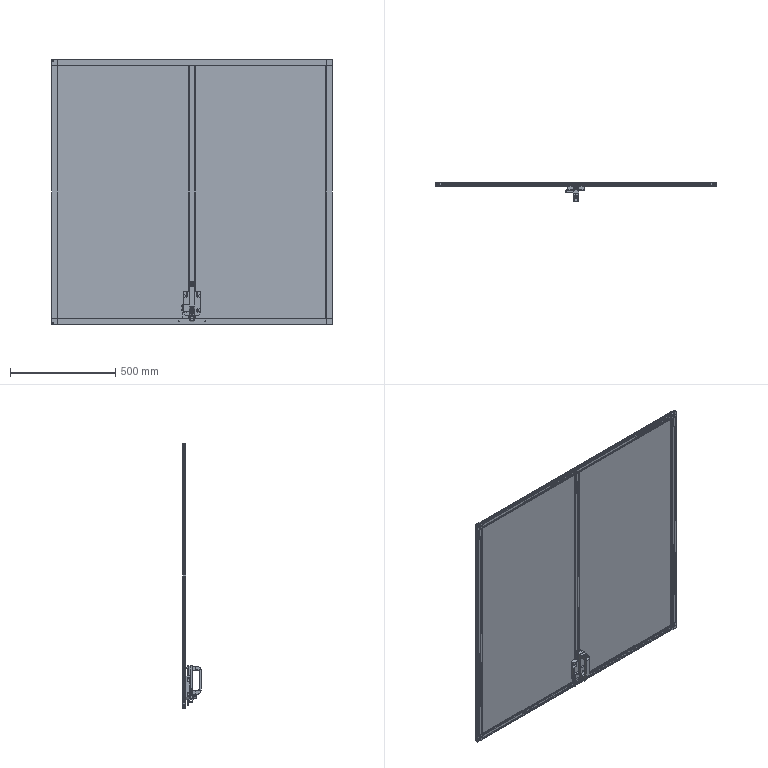Part | SolidWorks | features ReferencePattern 3, LocalLPattern 2 | 19 solids | 1717 faces | box 1336 x 89 x 1260 mm | volume 9587971 mm3 | plane 896 | cylinder 470 | cone 285 | spline 60 | torus 6 | commonest cylinder face diameters 5 x101 1 x86 11 x56 6 x24 2 x22 3.3 x20